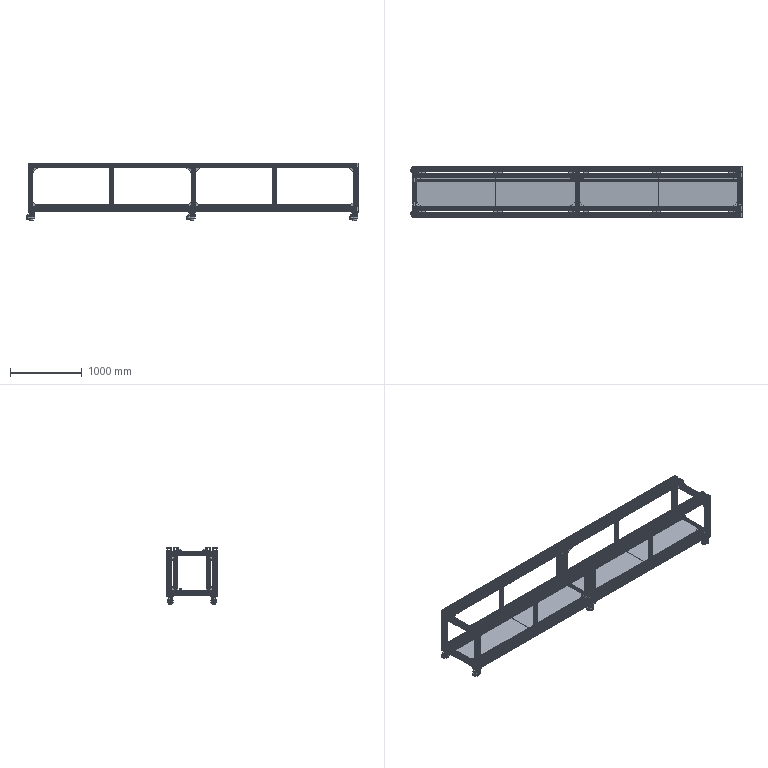Part | NX | features BREP 18 | 158 solids | 12560 faces | volume 79261005 mm3 | plane 7921 | cylinder 3779 | spline 416 | cone 312 | torus 132 | commonest cylinder face diameters 0.6 x736 6.8 x712 2 x492 6.6 x300 4 x286 8.2 x160